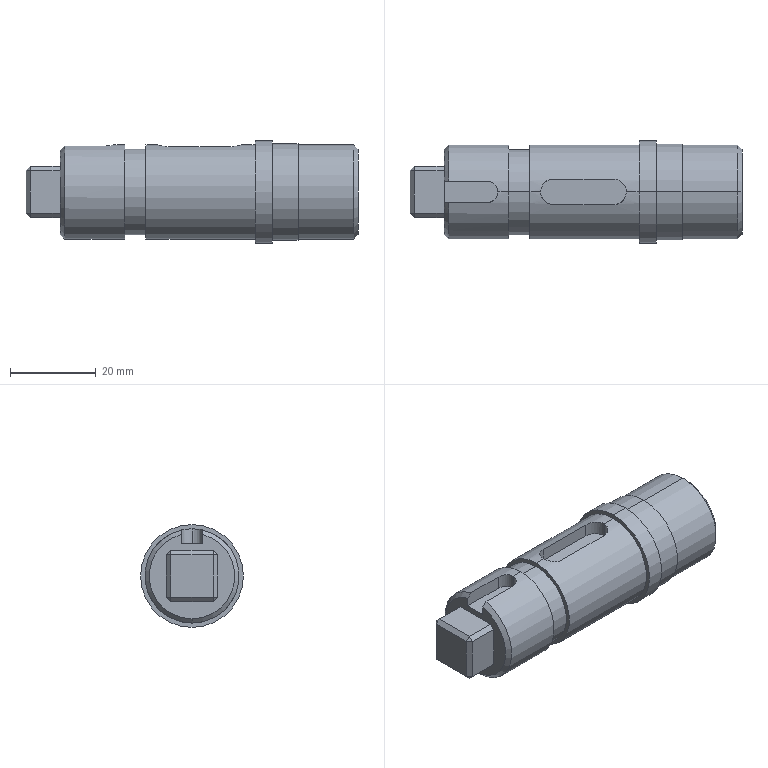Part | SolidWorks | features ICE 3, Chamfer 1, Revolution 1 | 1 solid | 51 faces | box 77.5 x 24 x 24 mm | volume 26951 mm3 | plane 30 | cylinder 17 | cone 4 | commonest cylinder face diameters 22 x6 6 x3 5 x2 20 x2 22.5 x2 24 x2
STEP:
#1=CARTESIAN_POINT('',(-28.866,0.,7.5));
#2=VERTEX_POINT('',#1);
#3=CARTESIAN_POINT('',(-31.366,2.5,7.5));
#4=VERTEX_POINT('',#3);
#5=CARTESIAN_POINT('',(-31.366,0.,7.5));
#6=DIRECTION('',(0.,0.,1.));
#7=DIRECTION('',(1.,0.,0.));
#8=AXIS2_PLACEMENT_3D('',#5,#6,#7);
#9=CIRCLE('',#8,2.5);
#10=EDGE_CURVE('',#2,#4,#9,.T.);
#11=ORIENTED_EDGE('',*,*,#10,.F.);
#12=CARTESIAN_POINT('',(-28.866,0.,11.));
#13=VERTEX_POINT('',#12);
#14=CARTESIAN_POINT('',(-28.866,0.,7.5));
#15=DIRECTION('',(0.,0.,1.));
#16=VECTOR('',#15,1000.);
#17=LINE('',#14,#16);
#18=EDGE_CURVE('',#2,#13,#17,.T.);
#19=ORIENTED_EDGE('',*,*,#18,.T.);
#20=CARTESIAN_POINT('',(-31.366,2.5,10.712));
#21=VERTEX_POINT('',#20);
#22=CARTESIAN_POINT('',(-31.366,2.5,10.712));
#23=CARTESIAN_POINT('',(-31.2,2.5,10.712));
#24=CARTESIAN_POINT('',(-31.037,2.484,10.716));
#25=CARTESIAN_POINT('',(-30.717,2.42,10.731));
#26=CARTESIAN_POINT('',(-30.558,2.371,10.742));
#27=CARTESIAN_POINT('',(-30.255,2.246,10.769));
#28=CARTESIAN_POINT('',(-30.112,2.169,10.784));
#29=CARTESIAN_POINT('',(-29.84,1.987,10.819));
#30=CARTESIAN_POINT('',(-29.712,1.882,10.838));
#31=CARTESIAN_POINT('',(-29.367,1.537,10.895));
#32=CARTESIAN_POINT('',(-29.181,1.259,10.932));
#33=CARTESIAN_POINT('',(-28.994,0.8077,10.971));
#34=CARTESIAN_POINT('',(-28.946,0.6494,10.982));
#35=CARTESIAN_POINT('',(-28.882,0.3264,10.996));
#36=CARTESIAN_POINT('',(-28.866,0.1637,11.));
#37=CARTESIAN_POINT('',(-28.866,0.,11.));
#38=B_SPLINE_CURVE_WITH_KNOTS('',3,(#22,#23,#24,#25,#26,#27,#28,#29,#30,#31,#32,#33,#34,#35,#36,#37),.UNSPECIFIED.,.F.,.F.,(4,2,2,2,2,2,2,4),(0.,0.0004902,0.0009805,0.001471,0.001961,0.002941,0.003432,0.003922),.UNSPECIFIED.);
#39=EDGE_CURVE('',#21,#13,#38,.T.);
#40=ORIENTED_EDGE('',*,*,#39,.F.);
#41=CARTESIAN_POINT('',(-31.366,2.5,7.5));
#42=DIRECTION('',(0.,0.,1.));
#43=VECTOR('',#42,1000.);
#44=LINE('',#41,#43);
#45=EDGE_CURVE('',#4,#21,#44,.T.);
#46=ORIENTED_EDGE('',*,*,#45,.F.);
#47=EDGE_LOOP('',(#11,#19,#40,#46));
#48=FACE_OUTER_BOUND('',#47,.T.);
#49=CARTESIAN_POINT('',(-31.366,0.,7.5));
#50=DIRECTION('',(0.,0.,1.));
#51=DIRECTION('',(1.,0.,0.));
#52=AXIS2_PLACEMENT_3D('',#49,#50,#51);
#53=CYLINDRICAL_SURFACE('',#52,2.5);
#54=ADVANCED_FACE('',(#48),#53,.F.);
#55=CARTESIAN_POINT('',(1.134,0.,7.5));
#56=VERTEX_POINT('',#55);
#57=CARTESIAN_POINT('',(-1.866,3.,7.5));
#58=VERTEX_POINT('',#57);
#59=CARTESIAN_POINT('',(-1.866,0.,7.5));
#60=DIRECTION('',(0.,0.,1.));
#61=DIRECTION('',(1.,0.,0.));
#62=AXIS2_PLACEMENT_3D('',#59,#60,#61);
#63=CIRCLE('',#62,3.);
#64=EDGE_CURVE('',#56,#58,#63,.T.);
#65=ORIENTED_EDGE('',*,*,#64,.F.);
#66=CARTESIAN_POINT('',(1.134,0.,11.));
#67=VERTEX_POINT('',#66);
#68=CARTESIAN_POINT('',(1.134,0.,7.5));
#69=DIRECTION('',(0.,0.,1.));
#70=VECTOR('',#69,1000.);
#71=LINE('',#68,#70);
#72=EDGE_CURVE('',#56,#67,#71,.T.);
#73=ORIENTED_EDGE('',*,*,#72,.T.);
#74=CARTESIAN_POINT('',(-1.866,3.,10.583));
#75=VERTEX_POINT('',#74);
#76=CARTESIAN_POINT('',(-1.866,3.,10.583));
#77=CARTESIAN_POINT('',(-1.666,3.,10.583));
#78=CARTESIAN_POINT('',(-1.471,2.98,10.589));
#79=CARTESIAN_POINT('',(-1.086,2.903,10.61));
#80=CARTESIAN_POINT('',(-0.8948,2.845,10.626));
#81=CARTESIAN_POINT('',(-0.5318,2.694,10.665));
#82=CARTESIAN_POINT('',(-0.3599,2.602,10.688));
#83=CARTESIAN_POINT('',(-0.03443,2.384,10.739));
#84=CARTESIAN_POINT('',(0.1189,2.258,10.767));
#85=CARTESIAN_POINT('',(0.3941,1.983,10.821));
#86=CARTESIAN_POINT('',(0.518,1.832,10.848));
#87=CARTESIAN_POINT('',(0.7374,1.504,10.898));
#88=CARTESIAN_POINT('',(0.8299,1.331,10.921));
#89=CARTESIAN_POINT('',(0.9797,0.9703,10.959));
#90=CARTESIAN_POINT('',(1.038,0.78,10.974));
#91=CARTESIAN_POINT('',(1.115,0.3922,10.995));
#92=CARTESIAN_POINT('',(1.134,0.1968,11.));
#93=CARTESIAN_POINT('',(1.134,0.,11.));
#94=B_SPLINE_CURVE_WITH_KNOTS('',3,(#76,#77,#78,#79,#80,#81,#82,#83,#84,#85,#86,#87,#88,#89,#90,#91,#92,#93),.UNSPECIFIED.,.F.,.F.,(4,2,2,2,2,2,2,2,4),(0.,0.0005892,0.001178,0.001767,0.002357,0.002946,0.003535,0.004124,0.004713),.UNSPECIFIED.);
#95=EDGE_CURVE('',#75,#67,#94,.T.);
#96=ORIENTED_EDGE('',*,*,#95,.F.);
#97=CARTESIAN_POINT('',(-1.866,3.,7.5));
#98=DIRECTION('',(0.,0.,1.));
#99=VECTOR('',#98,1000.);
#100=LINE('',#97,#99);
#101=EDGE_CURVE('',#58,#75,#100,.T.);
#102=ORIENTED_EDGE('',*,*,#101,.F.);
#103=EDGE_LOOP('',(#65,#73,#96,#102));
#104=FACE_OUTER_BOUND('',#103,.T.);
#105=CARTESIAN_POINT('',(-1.866,0.,7.5));
#106=DIRECTION('',(0.,0.,1.));
#107=DIRECTION('',(1.,0.,0.));
#108=AXIS2_PLACEMENT_3D('',#105,#106,#107);
#109=CYLINDRICAL_SURFACE('',#108,3.);
#110=ADVANCED_FACE('',(#104),#109,.F.);
#111=CARTESIAN_POINT('',(-41.366,0.,-10.));
#112=VERTEX_POINT('',#111);
#113=CARTESIAN_POINT('',(-41.366,-2.5,9.682));
#114=VERTEX_POINT('',#113);
#115=CARTESIAN_POINT('',(-41.366,0.,0.));
#116=DIRECTION('',(-1.,0.,0.));
#117=DIRECTION('',(0.,0.,-1.));
#118=AXIS2_PLACEMENT_3D('',#115,#116,#117);
#119=CIRCLE('',#118,10.);
#120=EDGE_CURVE('',#112,#114,#119,.T.);
#121=ORIENTED_EDGE('',*,*,#120,.F.);
#122=CARTESIAN_POINT('',(-40.366,0.,-11.));
#123=VERTEX_POINT('',#122);
#124=CARTESIAN_POINT('',(-41.366,0.,-10.));
#125=DIRECTION('',(0.7071,0.,-0.7071));
#126=VECTOR('',#125,1000.);
#127=LINE('',#124,#126);
#128=EDGE_CURVE('',#112,#123,#127,.T.);
#129=ORIENTED_EDGE('',*,*,#128,.T.);
#130=CARTESIAN_POINT('',(-40.366,-2.5,10.712));
#131=VERTEX_POINT('',#130);
#132=CARTESIAN_POINT('',(-40.366,0.,0.));
#133=DIRECTION('',(1.,0.,0.));
#134=DIRECTION('',(0.,0.,-1.));
#135=AXIS2_PLACEMENT_3D('',#132,#133,#134);
#136=CIRCLE('',#135,11.);
#137=EDGE_CURVE('',#131,#123,#136,.T.);
#138=ORIENTED_EDGE('',*,*,#137,.F.);
#139=CARTESIAN_POINT('',(-41.366,-2.5,9.682));
#140=CARTESIAN_POINT('',(-41.033,-2.5,10.026));
#141=CARTESIAN_POINT('',(-40.7,-2.5,10.369));
#142=CARTESIAN_POINT('',(-40.366,-2.5,10.712));
#143=B_SPLINE_CURVE_WITH_KNOTS('',3,(#139,#140,#141,#142),.UNSPECIFIED.,.F.,.F.,(4,4),(0.005287,0.006723),.UNSPECIFIED.);
#144=EDGE_CURVE('',#114,#131,#143,.T.);
#145=ORIENTED_EDGE('',*,*,#144,.F.);
#146=EDGE_LOOP('',(#121,#129,#138,#145));
#147=FACE_OUTER_BOUND('',#146,.T.);
#148=CARTESIAN_POINT('',(-41.366,0.,0.));
#149=DIRECTION('',(1.,0.,0.));
#150=DIRECTION('',(0.,0.,-1.));
#151=AXIS2_PLACEMENT_3D('',#148,#149,#150);
#152=CONICAL_SURFACE('',#151,10.,0.7854);
#153=ADVANCED_FACE('',(#147),#152,.T.);
#154=CARTESIAN_POINT('',(28.134,0.,-10.));
#155=VERTEX_POINT('',#154);
#156=CARTESIAN_POINT('',(28.134,0.,10.));
#157=VERTEX_POINT('',#156);
#158=CARTESIAN_POINT('',(28.134,0.,0.));
#159=DIRECTION('',(1.,0.,0.));
#160=DIRECTION('',(0.,0.,1.));
#161=AXIS2_PLACEMENT_3D('',#158,#159,#160);
#162=CIRCLE('',#161,10.);
#163=EDGE_CURVE('',#155,#157,#162,.T.);
#164=ORIENTED_EDGE('',*,*,#163,.F.);
#165=CARTESIAN_POINT('',(27.134,0.,-11.));
#166=VERTEX_POINT('',#165);
#167=CARTESIAN_POINT('',(27.134,0.,-11.));
#168=DIRECTION('',(-0.7071,0.,-0.7071));
#169=VECTOR('',#168,1000.);
#170=LINE('',#167,#169);
#171=EDGE_CURVE('',#155,#166,#170,.T.);
#172=ORIENTED_EDGE('',*,*,#171,.T.);
#173=CARTESIAN_POINT('',(27.134,0.,11.));
#174=VERTEX_POINT('',#173);
#175=CARTESIAN_POINT('',(27.134,0.,0.));
#176=DIRECTION('',(-1.,0.,0.));
#177=DIRECTION('',(0.,0.,1.));
#178=AXIS2_PLACEMENT_3D('',#175,#176,#177);
#179=CIRCLE('',#178,11.);
#180=EDGE_CURVE('',#174,#166,#179,.T.);
#181=ORIENTED_EDGE('',*,*,#180,.F.);
#182=CARTESIAN_POINT('',(27.134,0.,11.));
#183=DIRECTION('',(-0.7071,0.,0.7071));
#184=VECTOR('',#183,1000.);
#185=LINE('',#182,#184);
#186=EDGE_CURVE('',#157,#174,#185,.T.);
#187=ORIENTED_EDGE('',*,*,#186,.F.);
#188=EDGE_LOOP('',(#164,#172,#181,#187));
#189=FACE_OUTER_BOUND('',#188,.T.);
#190=CARTESIAN_POINT('',(27.134,0.,0.));
#191=DIRECTION('',(-1.,0.,0.));
#192=DIRECTION('',(0.,0.,1.));
#193=AXIS2_PLACEMENT_3D('',#190,#191,#192);
#194=CONICAL_SURFACE('',#193,11.,0.7854);
#195=ADVANCED_FACE('',(#189),#194,.T.);
#196=CARTESIAN_POINT('',(-26.366,0.,11.));
#197=VERTEX_POINT('',#196);
#198=CARTESIAN_POINT('',(-26.366,0.,-11.));
#199=VERTEX_POINT('',#198);
#200=CARTESIAN_POINT('',(-26.366,0.,0.));
#201=DIRECTION('',(-1.,0.,0.));
#202=DIRECTION('',(0.,0.,1.));
#203=AXIS2_PLACEMENT_3D('',#200,#201,#202);
#204=CIRCLE('',#203,11.);
#205=EDGE_CURVE('',#197,#199,#204,.T.);
#206=ORIENTED_EDGE('',*,*,#205,.T.);
#207=CARTESIAN_POINT('',(-41.366,0.,-11.));
#208=DIRECTION('',(-1.,0.,0.));
#209=VECTOR('',#208,1000.);
#210=LINE('',#207,#209);
#211=EDGE_CURVE('',#199,#123,#210,.T.);
#212=ORIENTED_EDGE('',*,*,#211,.T.);
#213=CARTESIAN_POINT('',(-40.366,2.5,10.712));
#214=VERTEX_POINT('',#213);
#215=CARTESIAN_POINT('',(-40.366,0.,0.));
#216=DIRECTION('',(1.,0.,0.));
#217=DIRECTION('',(0.,0.,-1.));
#218=AXIS2_PLACEMENT_3D('',#215,#216,#217);
#219=CIRCLE('',#218,11.);
#220=EDGE_CURVE('',#123,#214,#219,.T.);
#221=ORIENTED_EDGE('',*,*,#220,.T.);
#222=CARTESIAN_POINT('',(-41.366,2.5,10.712));
#223=DIRECTION('',(1.,0.,0.));
#224=VECTOR('',#223,1000.);
#225=LINE('',#222,#224);
#226=EDGE_CURVE('',#214,#21,#225,.T.);
#227=ORIENTED_EDGE('',*,*,#226,.T.);
#228=ORIENTED_EDGE('',*,*,#39,.T.);
#229=CARTESIAN_POINT('',(-41.366,0.,11.));
#230=DIRECTION('',(-1.,0.,0.));
#231=VECTOR('',#230,1000.);
#232=LINE('',#229,#231);
#233=EDGE_CURVE('',#197,#13,#232,.T.);
#234=ORIENTED_EDGE('',*,*,#233,.F.);
#235=EDGE_LOOP('',(#206,#212,#221,#227,#228,#234));
#236=FACE_OUTER_BOUND('',#235,.T.);
#237=CARTESIAN_POINT('',(-41.366,0.,0.));
#238=DIRECTION('',(-1.,0.,0.));
#239=DIRECTION('',(0.,0.,1.));
#240=AXIS2_PLACEMENT_3D('',#237,#238,#239);
#241=CYLINDRICAL_SURFACE('',#240,11.);
#242=ADVANCED_FACE('',(#236),#241,.T.);
#243=CARTESIAN_POINT('',(-21.366,0.,10.));
#244=VERTEX_POINT('',#243);
#245=CARTESIAN_POINT('',(-21.366,0.,-10.));
#246=VERTEX_POINT('',#245);
#247=CARTESIAN_POINT('',(-21.366,0.,0.));
#248=DIRECTION('',(-1.,0.,0.));
#249=DIRECTION('',(0.,0.,1.));
#250=AXIS2_PLACEMENT_3D('',#247,#248,#249);
#251=CIRCLE('',#250,10.);
#252=EDGE_CURVE('',#244,#246,#251,.T.);
#253=ORIENTED_EDGE('',*,*,#252,.T.);
#254=CARTESIAN_POINT('',(-26.366,0.,-10.));
#255=VERTEX_POINT('',#254);
#256=CARTESIAN_POINT('',(-41.366,0.,-10.));
#257=DIRECTION('',(-1.,0.,0.));
#258=VECTOR('',#257,1000.);
#259=LINE('',#256,#258);
#260=EDGE_CURVE('',#246,#255,#259,.T.);
#261=ORIENTED_EDGE('',*,*,#260,.T.);
#262=CARTESIAN_POINT('',(-26.366,0.,10.));
#263=VERTEX_POINT('',#262);
#264=CARTESIAN_POINT('',(-26.366,0.,0.));
#265=DIRECTION('',(-1.,0.,0.));
#266=DIRECTION('',(0.,0.,1.));
#267=AXIS2_PLACEMENT_3D('',#264,#265,#266);
#268=CIRCLE('',#267,10.);
#269=EDGE_CURVE('',#263,#255,#268,.T.);
#270=ORIENTED_EDGE('',*,*,#269,.F.);
#271=CARTESIAN_POINT('',(-41.366,0.,10.));
#272=DIRECTION('',(-1.,0.,0.));
#273=VECTOR('',#272,1000.);
#274=LINE('',#271,#273);
#275=EDGE_CURVE('',#244,#263,#274,.T.);
#276=ORIENTED_EDGE('',*,*,#275,.F.);
#277=EDGE_LOOP('',(#253,#261,#270,#276));
#278=FACE_OUTER_BOUND('',#277,.T.);
#279=CARTESIAN_POINT('',(-41.366,0.,0.));
#280=DIRECTION('',(-1.,0.,0.));
#281=DIRECTION('',(0.,0.,1.));
#282=AXIS2_PLACEMENT_3D('',#279,#280,#281);
#283=CYLINDRICAL_SURFACE('',#282,10.);
#284=ADVANCED_FACE('',(#278),#283,.T.);
#285=CARTESIAN_POINT('',(4.134,0.,11.));
#286=VERTEX_POINT('',#285);
#287=CARTESIAN_POINT('',(4.134,0.,-11.));
#288=VERTEX_POINT('',#287);
#289=CARTESIAN_POINT('',(4.134,0.,0.));
#290=DIRECTION('',(-1.,0.,0.));
#291=DIRECTION('',(0.,0.,1.));
#292=AXIS2_PLACEMENT_3D('',#289,#290,#291);
#293=CIRCLE('',#292,11.);
#294=EDGE_CURVE('',#286,#288,#293,.T.);
#295=ORIENTED_EDGE('',*,*,#294,.T.);
#296=CARTESIAN_POINT('',(-21.366,0.,-11.));
#297=VERTEX_POINT('',#296);
#298=CARTESIAN_POINT('',(-41.366,0.,-11.));
#299=DIRECTION('',(-1.,0.,0.));
#300=VECTOR('',#299,1000.);
#301=LINE('',#298,#300);
#302=EDGE_CURVE('',#288,#297,#301,.T.);
#303=ORIENTED_EDGE('',*,*,#302,.T.);
#304=CARTESIAN_POINT('',(-21.366,0.,11.));
#305=VERTEX_POINT('',#304);
#306=CARTESIAN_POINT('',(-21.366,0.,0.));
#307=DIRECTION('',(-1.,0.,0.));
#308=DIRECTION('',(0.,0.,1.));
#309=AXIS2_PLACEMENT_3D('',#306,#307,#308);
#310=CIRCLE('',#309,11.);
#311=EDGE_CURVE('',#305,#297,#310,.T.);
#312=ORIENTED_EDGE('',*,*,#311,.F.);
#313=CARTESIAN_POINT('',(-18.866,0.,11.));
#314=VERTEX_POINT('',#313);
#315=CARTESIAN_POINT('',(-41.366,0.,11.));
#316=DIRECTION('',(-1.,0.,0.));
#317=VECTOR('',#316,1000.);
#318=LINE('',#315,#317);
#319=EDGE_CURVE('',#314,#305,#318,.T.);
#320=ORIENTED_EDGE('',*,*,#319,.F.);
#321=CARTESIAN_POINT('',(-15.866,3.,10.583));
#322=VERTEX_POINT('',#321);
#323=CARTESIAN_POINT('',(-18.866,0.,11.));
#324=CARTESIAN_POINT('',(-18.866,0.1966,11.));
#325=CARTESIAN_POINT('',(-18.846,0.3963,10.995));
#326=CARTESIAN_POINT('',(-18.769,0.7814,10.974));
#327=CARTESIAN_POINT('',(-18.712,0.9688,10.959));
#328=CARTESIAN_POINT('',(-18.485,1.515,10.901));
#329=CARTESIAN_POINT('',(-18.264,1.844,10.848));
#330=CARTESIAN_POINT('',(-17.848,2.26,10.766));
#331=CARTESIAN_POINT('',(-17.698,2.383,10.739));
#332=CARTESIAN_POINT('',(-17.374,2.601,10.689));
#333=CARTESIAN_POINT('',(-17.199,2.695,10.665));
#334=CARTESIAN_POINT('',(-16.837,2.845,10.626));
#335=CARTESIAN_POINT('',(-16.65,2.902,10.61));
#336=CARTESIAN_POINT('',(-16.264,2.98,10.589));
#337=CARTESIAN_POINT('',(-16.065,3.,10.583));
#338=CARTESIAN_POINT('',(-15.866,3.,10.583));
#339=B_SPLINE_CURVE_WITH_KNOTS('',3,(#323,#324,#325,#326,#327,#328,#329,#330,#331,#332,#333,#334,#335,#336,#337,#338),.UNSPECIFIED.,.F.,.F.,(4,2,2,2,2,2,2,4),(0.004713,0.005302,0.00589,0.007067,0.007656,0.008244,0.008833,0.009421),.UNSPECIFIED.);
#340=EDGE_CURVE('',#314,#322,#339,.T.);
#341=ORIENTED_EDGE('',*,*,#340,.T.);
#342=CARTESIAN_POINT('',(-41.366,3.,10.583));
#343=DIRECTION('',(1.,0.,0.));
#344=VECTOR('',#343,1000.);
#345=LINE('',#342,#344);
#346=EDGE_CURVE('',#322,#75,#345,.T.);
#347=ORIENTED_EDGE('',*,*,#346,.T.);
#348=ORIENTED_EDGE('',*,*,#95,.T.);
#349=CARTESIAN_POINT('',(-41.366,0.,11.));
#350=DIRECTION('',(-1.,0.,0.));
#351=VECTOR('',#350,1000.);
#352=LINE('',#349,#351);
#353=EDGE_CURVE('',#286,#67,#352,.T.);
#354=ORIENTED_EDGE('',*,*,#353,.F.);
#355=EDGE_LOOP('',(#295,#303,#312,#320,#341,#347,#348,#354));
#356=FACE_OUTER_BOUND('',#355,.T.);
#357=CARTESIAN_POINT('',(-41.366,0.,0.));
#358=DIRECTION('',(-1.,0.,0.));
#359=DIRECTION('',(0.,0.,1.));
#360=AXIS2_PLACEMENT_3D('',#357,#358,#359);
#361=CYLINDRICAL_SURFACE('',#360,11.);
#362=ADVANCED_FACE('',(#356),#361,.T.);
#363=CARTESIAN_POINT('',(8.134,0.,12.));
#364=VERTEX_POINT('',#363);
#365=CARTESIAN_POINT('',(8.134,0.,-12.));
#366=VERTEX_POINT('',#365);
#367=CARTESIAN_POINT('',(8.134,0.,0.));
#368=DIRECTION('',(-1.,0.,0.));
#369=DIRECTION('',(0.,0.,1.));
#370=AXIS2_PLACEMENT_3D('',#367,#368,#369);
#371=CIRCLE('',#370,12.);
#372=EDGE_CURVE('',#364,#366,#371,.T.);
#373=ORIENTED_EDGE('',*,*,#372,.T.);
#374=CARTESIAN_POINT('',(4.134,0.,-12.));
#375=VERTEX_POINT('',#374);
#376=CARTESIAN_POINT('',(-41.366,0.,-12.));
#377=DIRECTION('',(-1.,0.,0.));
#378=VECTOR('',#377,1000.);
#379=LINE('',#376,#378);
#380=EDGE_CURVE('',#366,#375,#379,.T.);
#381=ORIENTED_EDGE('',*,*,#380,.T.);
#382=CARTESIAN_POINT('',(4.134,0.,12.));
#383=VERTEX_POINT('',#382);
#384=CARTESIAN_POINT('',(4.134,0.,0.));
#385=DIRECTION('',(-1.,0.,0.));
#386=DIRECTION('',(0.,0.,1.));
#387=AXIS2_PLACEMENT_3D('',#384,#385,#386);
#388=CIRCLE('',#387,12.);
#389=EDGE_CURVE('',#383,#375,#388,.T.);
#390=ORIENTED_EDGE('',*,*,#389,.F.);
#391=CARTESIAN_POINT('',(-41.366,0.,12.));
#392=DIRECTION('',(-1.,0.,0.));
#393=VECTOR('',#392,1000.);
#394=LINE('',#391,#393);
#395=EDGE_CURVE('',#364,#383,#394,.T.);
#396=ORIENTED_EDGE('',*,*,#395,.F.);
#397=EDGE_LOOP('',(#373,#381,#390,#396));
#398=FACE_OUTER_BOUND('',#397,.T.);
#399=CARTESIAN_POINT('',(-41.366,0.,0.));
#400=DIRECTION('',(-1.,0.,0.));
#401=DIRECTION('',(0.,0.,1.));
#402=AXIS2_PLACEMENT_3D('',#399,#400,#401);
#403=CYLINDRICAL_SURFACE('',#402,12.);
#404=ADVANCED_FACE('',(#398),#403,.T.);
#405=CARTESIAN_POINT('',(14.134,0.,11.25));
#406=VERTEX_POINT('',#405);
#407=CARTESIAN_POINT('',(14.134,0.,-11.25));
#408=VERTEX_POINT('',#407);
#409=CARTESIAN_POINT('',(14.134,0.,0.));
#410=DIRECTION('',(-1.,0.,0.));
#411=DIRECTION('',(0.,0.,1.));
#412=AXIS2_PLACEMENT_3D('',#409,#410,#411);
#413=CIRCLE('',#412,11.25);
#414=EDGE_CURVE('',#406,#408,#413,.T.);
#415=ORIENTED_EDGE('',*,*,#414,.T.);
#416=CARTESIAN_POINT('',(8.134,0.,-11.25));
#417=VERTEX_POINT('',#416);
#418=CARTESIAN_POINT('',(-41.366,0.,-11.25));
#419=DIRECTION('',(-1.,0.,0.));
#420=VECTOR('',#419,1000.);
#421=LINE('',#418,#420);
#422=EDGE_CURVE('',#408,#417,#421,.T.);
#423=ORIENTED_EDGE('',*,*,#422,.T.);
#424=CARTESIAN_POINT('',(8.134,0.,11.25));
#425=VERTEX_POINT('',#424);
#426=CARTESIAN_POINT('',(8.134,0.,0.));
#427=DIRECTION('',(-1.,0.,0.));
#428=DIRECTION('',(0.,0.,1.));
#429=AXIS2_PLACEMENT_3D('',#426,#427,#428);
#430=CIRCLE('',#429,11.25);
#431=EDGE_CURVE('',#425,#417,#430,.T.);
#432=ORIENTED_EDGE('',*,*,#431,.F.);
#433=CARTESIAN_POINT('',(-41.366,0.,11.25));
#434=DIRECTION('',(-1.,0.,0.));
#435=VECTOR('',#434,1000.);
#436=LINE('',#433,#435);
#437=EDGE_CURVE('',#406,#425,#436,.T.);
#438=ORIENTED_EDGE('',*,*,#437,.F.);
#439=EDGE_LOOP('',(#415,#423,#432,#438));
#440=FACE_OUTER_BOUND('',#439,.T.);
#441=CARTESIAN_POINT('',(-41.366,0.,0.));
#442=DIRECTION('',(-1.,0.,0.));
#443=DIRECTION('',(0.,0.,1.));
#444=AXIS2_PLACEMENT_3D('',#441,#442,#443);
#445=CYLINDRICAL_SURFACE('',#444,11.25);
#446=ADVANCED_FACE('',(#440),#445,.T.);
#447=ORIENTED_EDGE('',*,*,#180,.T.);
#448=CARTESIAN_POINT('',(14.134,0.,-11.));
#449=VERTEX_POINT('',#448);
#450=CARTESIAN_POINT('',(-41.366,0.,-11.));
#451=DIRECTION('',(-1.,0.,0.));
#452=VECTOR('',#451,1000.);
#453=LINE('',#450,#452);
#454=EDGE_CURVE('',#166,#449,#453,.T.);
#455=ORIENTED_EDGE('',*,*,#454,.T.);
#456=CARTESIAN_POINT('',(14.134,0.,11.));
#457=VERTEX_POINT('',#456);
#458=CARTESIAN_POINT('',(14.134,0.,0.));
#459=DIRECTION('',(-1.,0.,0.));
#460=DIRECTION('',(0.,0.,1.));
#461=AXIS2_PLACEMENT_3D('',#458,#459,#460);
#462=CIRCLE('',#461,11.);
#463=EDGE_CURVE('',#457,#449,#462,.T.);
#464=ORIENTED_EDGE('',*,*,#463,.F.);
#465=CARTESIAN_POINT('',(-41.366,0.,11.));
#466=DIRECTION('',(-1.,0.,0.));
#467=VECTOR('',#466,1000.);
#468=LINE('',#465,#467);
#469=EDGE_CURVE('',#174,#457,#468,.T.);
#470=ORIENTED_EDGE('',*,*,#469,.F.);
#471=EDGE_LOOP('',(#447,#455,#464,#470));
#472=FACE_OUTER_BOUND('',#471,.T.);
#473=CARTESIAN_POINT('',(-41.366,0.,0.));
#474=DIRECTION('',(-1.,0.,0.));
#475=DIRECTION('',(0.,0.,1.));
#476=AXIS2_PLACEMENT_3D('',#473,#474,#475);
#477=CYLINDRICAL_SURFACE('',#476,11.);
#478=ADVANCED_FACE('',(#472),#477,.T.);
#479=CARTESIAN_POINT('',(-41.366,2.5,9.682));
#480=VERTEX_POINT('',#479);
#481=CARTESIAN_POINT('',(-41.366,0.,0.));
#482=DIRECTION('',(-1.,0.,0.));
#483=DIRECTION('',(0.,0.,-1.));
#484=AXIS2_PLACEMENT_3D('',#481,#482,#483);
#485=CIRCLE('',#484,10.);
#486=EDGE_CURVE('',#480,#112,#485,.T.);
#487=ORIENTED_EDGE('',*,*,#486,.T.);
#488=ORIENTED_EDGE('',*,*,#120,.T.);
#489=CARTESIAN_POINT('',(-41.366,-2.5,7.5));
#490=VERTEX_POINT('',#489);
#491=CARTESIAN_POINT('',(-41.366,-2.5,7.5));
#492=DIRECTION('',(0.,0.,1.));
#493=VECTOR('',#492,1000.);
#494=LINE('',#491,#493);
#495=EDGE_CURVE('',#490,#114,#494,.T.);
#496=ORIENTED_EDGE('',*,*,#495,.F.);
#497=CARTESIAN_POINT('',(-41.366,2.5,7.5));
#498=VERTEX_POINT('',#497);
#499=CARTESIAN_POINT('',(-41.366,2.5,7.5));
#500=DIRECTION('',(0.,-1.,0.));
#501=VECTOR('',#500,1000.);
#502=LINE('',#499,#501);
#503=EDGE_CURVE('',#498,#490,#502,.T.);
#504=ORIENTED_EDGE('',*,*,#503,.F.);
#505=CARTESIAN_POINT('',(-41.366,2.5,7.5));
#506=DIRECTION('',(0.,0.,1.));
#507=VECTOR('',#506,1000.);
#508=LINE('',#505,#507);
#509=EDGE_CURVE('',#498,#480,#508,.T.);
#510=ORIENTED_EDGE('',*,*,#509,.T.);
#511=EDGE_LOOP('',(#487,#488,#496,#504,#510));
#512=FACE_OUTER_BOUND('',#511,.T.);
#513=CARTESIAN_POINT('',(-41.366,-5.,6.));
#514=VERTEX_POINT('',#513);
#515=CARTESIAN_POINT('',(-41.366,5.,6.));
#516=VERTEX_POINT('',#515);
#517=CARTESIAN_POINT('',(-41.366,-6.,6.));
#518=DIRECTION('',(0.,1.,0.));
#519=VECTOR('',#518,1000.);
#520=LINE('',#517,#519);
#521=EDGE_CURVE('',#514,#516,#520,.T.);
#522=ORIENTED_EDGE('',*,*,#521,.F.);
#523=CARTESIAN_POINT('',(-41.366,-6.,5.));
#524=VERTEX_POINT('',#523);
#525=CARTESIAN_POINT('',(-41.366,0.,11.));
#526=DIRECTION('',(0.,-0.7071,-0.7071));
#527=VECTOR('',#526,1000.);
#528=LINE('',#525,#527);
#529=EDGE_CURVE('',#514,#524,#528,.T.);
#530=ORIENTED_EDGE('',*,*,#529,.T.);
#531=CARTESIAN_POINT('',(-41.366,-6.,-5.));
#532=VERTEX_POINT('',#531);
#533=CARTESIAN_POINT('',(-41.366,-6.,-6.));
#534=DIRECTION('',(0.,0.,1.));
#535=VECTOR('',#534,1000.);
#536=LINE('',#533,#535);
#537=EDGE_CURVE('',#532,#524,#536,.T.);
#538=ORIENTED_EDGE('',*,*,#537,.F.);
#539=CARTESIAN_POINT('',(-41.366,-5.,-6.));
#540=VERTEX_POINT('',#539);
#541=CARTESIAN_POINT('',(-41.366,0.,-11.));
#542=DIRECTION('',(0.,0.7071,-0.7071));
#543=VECTOR('',#542,1000.);
#544=LINE('',#541,#543);
#545=EDGE_CURVE('',#532,#540,#544,.T.);
#546=ORIENTED_EDGE('',*,*,#545,.T.);
#547=CARTESIAN_POINT('',(-41.366,5.,-6.));
#548=VERTEX_POINT('',#547);
#549=CARTESIAN_POINT('',(-41.366,-6.,-6.));
#550=DIRECTION('',(0.,-1.,0.));
#551=VECTOR('',#550,1000.);
#552=LINE('',#549,#551);
#553=EDGE_CURVE('',#548,#540,#552,.T.);
#554=ORIENTED_EDGE('',*,*,#553,.F.);
#555=CARTESIAN_POINT('',(-41.366,6.,-5.));
#556=VERTEX_POINT('',#555);
#557=CARTESIAN_POINT('',(-41.366,11.,0.));
#558=DIRECTION('',(0.,0.7071,0.7071));
#559=VECTOR('',#558,1000.);
#560=LINE('',#557,#559);
#561=EDGE_CURVE('',#548,#556,#560,.T.);
#562=ORIENTED_EDGE('',*,*,#561,.T.);
#563=CARTESIAN_POINT('',(-41.366,6.,5.));
#564=VERTEX_POINT('',#563);
#565=CARTESIAN_POINT('',(-41.366,6.,-6.));
#566=DIRECTION('',(0.,0.,-1.));
#567=VECTOR('',#566,1000.);
#568=LINE('',#565,#567);
#569=EDGE_CURVE('',#564,#556,#568,.T.);
#570=ORIENTED_EDGE('',*,*,#569,.F.);
#571=CARTESIAN_POINT('',(-41.366,11.,0.));
#572=DIRECTION('',(0.,-0.7071,0.7071));
#573=VECTOR('',#572,1000.);
#574=LINE('',#571,#573);
#575=EDGE_CURVE('',#564,#516,#574,.T.);
#576=ORIENTED_EDGE('',*,*,#575,.T.);
#577=EDGE_LOOP('',(#522,#530,#538,#546,#554,#562,#570,#576));
#578=FACE_BOUND('',#577,.T.);
#579=CARTESIAN_POINT('',(-41.366,11.,0.));
#580=DIRECTION('',(1.,0.,0.));
#581=DIRECTION('',(0.,0.,-1.));
#582=AXIS2_PLACEMENT_3D('',#579,#580,#581);
#583=PLANE('',#582);
#584=ADVANCED_FACE('',(#512,#578),#583,.F.);
#585=CARTESIAN_POINT('',(28.134,0.,0.));
#586=DIRECTION('',(1.,0.,0.));
#587=DIRECTION('',(0.,0.,1.));
#588=AXIS2_PLACEMENT_3D('',#585,#586,#587);
#589=CIRCLE('',#588,10.);
#590=EDGE_CURVE('',#157,#155,#589,.T.);
#591=ORIENTED_EDGE('',*,*,#590,.T.);
#592=ORIENTED_EDGE('',*,*,#163,.T.);
#593=EDGE_LOOP('',(#591,#592));
#594=FACE_OUTER_BOUND('',#593,.T.);
#595=CARTESIAN_POINT('',(28.134,0.,0.));
#596=DIRECTION('',(-1.,0.,0.));
#597=DIRECTION('',(0.,0.,1.));
#598=AXIS2_PLACEMENT_3D('',#595,#596,#597);
#599=PLANE('',#598);
#600=ADVANCED_FACE('',(#594),#599,.F.);
#601=ORIENTED_EDGE('',*,*,#454,.F.);
#602=CARTESIAN_POINT('',(27.134,0.,0.));
#603=DIRECTION('',(-1.,0.,0.));
#604=DIRECTION('',(0.,0.,1.));
#605=AXIS2_PLACEMENT_3D('',#602,#603,#604);
#606=CIRCLE('',#605,11.);
#607=EDGE_CURVE('',#166,#174,#606,.T.);
#608=ORIENTED_EDGE('',*,*,#607,.T.);
#609=ORIENTED_EDGE('',*,*,#469,.T.);
#610=CARTESIAN_POINT('',(14.134,0.,0.));
#611=DIRECTION('',(-1.,0.,0.));
#612=DIRECTION('',(0.,0.,1.));
#613=AXIS2_PLACEMENT_3D('',#610,#611,#612);
#614=CIRCLE('',#613,11.);
#615=EDGE_CURVE('',#449,#457,#614,.T.);
#616=ORIENTED_EDGE('',*,*,#615,.F.);
#617=EDGE_LOOP('',(#601,#608,#609,#616));
#618=FACE_OUTER_BOUND('',#617,.T.);
#619=CARTESIAN_POINT('',(-41.366,0.,0.));
#620=DIRECTION('',(-1.,0.,0.));
#621=DIRECTION('',(0.,0.,1.));
#622=AXIS2_PLACEMENT_3D('',#619,#620,#621);
#623=CYLINDRICAL_SURFACE('',#622,11.);
#624=ADVANCED_FACE('',(#618),#623,.T.);
#625=ORIENTED_EDGE('',*,*,#414,.F.);
#626=CARTESIAN_POINT('',(14.134,0.,0.));
#627=DIRECTION('',(-1.,0.,0.));
#628=DIRECTION('',(0.,0.,1.));
#629=AXIS2_PLACEMENT_3D('',#626,#627,#628);
#630=CIRCLE('',#629,11.25);
#631=EDGE_CURVE('',#408,#406,#630,.T.);
#632=ORIENTED_EDGE('',*,*,#631,.F.);
#633=EDGE_LOOP('',(#625,#632));
#634=FACE_OUTER_BOUND('',#633,.T.);
#635=ORIENTED_EDGE('',*,*,#463,.T.);
#636=ORIENTED_EDGE('',*,*,#615,.T.);
#637=EDGE_LOOP('',(#635,#636));
#638=FACE_BOUND('',#637,.T.);
#639=CARTESIAN_POINT('',(14.134,11.,0.));
#640=DIRECTION('',(-1.,0.,0.));
#641=DIRECTION('',(0.,0.,1.));
#642=AXIS2_PLACEMENT_3D('',#639,#640,#641);
#643=PLANE('',#642);
#644=ADVANCED_FACE('',(#634,#638),#643,.F.);
#645=ORIENTED_EDGE('',*,*,#422,.F.);
#646=ORIENTED_EDGE('',*,*,#631,.T.);
#647=ORIENTED_EDGE('',*,*,#437,.T.);
#648=CARTESIAN_POINT('',(8.134,0.,0.));
#649=DIRECTION('',(-1.,0.,0.));
#650=DIRECTION('',(0.,0.,1.));
#651=AXIS2_PLACEMENT_3D('',#648,#649,#650);
#652=CIRCLE('',#651,11.25);
#653=EDGE_CURVE('',#417,#425,#652,.T.);
#654=ORIENTED_EDGE('',*,*,#653,.F.);
#655=EDGE_LOOP('',(#645,#646,#647,#654));
#656=FACE_OUTER_BOUND('',#655,.T.);
#657=CARTESIAN_POINT('',(-41.366,0.,0.));
#658=DIRECTION('',(-1.,0.,0.));
#659=DIRECTION('',(0.,0.,1.));
#660=AXIS2_PLACEMENT_3D('',#657,#658,#659);
#661=CYLINDRICAL_SURFACE('',#660,11.25);
#662=ADVANCED_FACE('',(#656),#661,.T.);
#663=ORIENTED_EDGE('',*,*,#372,.F.);
#664=CARTESIAN_POINT('',(8.134,0.,0.));
#665=DIRECTION('',(-1.,0.,0.));
#666=DIRECTION('',(0.,0.,1.));
#667=AXIS2_PLACEMENT_3D('',#664,#665,#666);
#668=CIRCLE('',#667,12.);
#669=EDGE_CURVE('',#366,#364,#668,.T.);
#670=ORIENTED_EDGE('',*,*,#669,.F.);
#671=EDGE_LOOP('',(#663,#670));
#672=FACE_OUTER_BOUND('',#671,.T.);
#673=ORIENTED_EDGE('',*,*,#431,.T.);
#674=ORIENTED_EDGE('',*,*,#653,.T.);
#675=EDGE_LOOP('',(#673,#674));
#676=FACE_BOUND('',#675,.T.);
#677=CARTESIAN_POINT('',(8.134,11.25,0.));
#678=DIRECTION('',(-1.,0.,0.));
#679=DIRECTION('',(0.,0.,1.));
#680=AXIS2_PLACEMENT_3D('',#677,#678,#679);
#681=PLANE('',#680);
#682=ADVANCED_FACE('',(#672,#676),#681,.F.);
#683=ORIENTED_EDGE('',*,*,#380,.F.);
#684=ORIENTED_EDGE('',*,*,#669,.T.);
#685=ORIENTED_EDGE('',*,*,#395,.T.);
#686=CARTESIAN_POINT('',(4.134,0.,0.));
#687=DIRECTION('',(-1.,0.,0.));
#688=DIRECTION('',(0.,0.,1.));
#689=AXIS2_PLACEMENT_3D('',#686,#687,#688);
#690=CIRCLE('',#689,12.);
#691=EDGE_CURVE('',#375,#383,#690,.T.);
#692=ORIENTED_EDGE('',*,*,#691,.F.);
#693=EDGE_LOOP('',(#683,#684,#685,#692));
#694=FACE_OUTER_BOUND('',#693,.T.);
#695=CARTESIAN_POINT('',(-41.366,0.,0.));
#696=DIRECTION('',(-1.,0.,0.));
#697=DIRECTION('',(0.,0.,1.));
#698=AXIS2_PLACEMENT_3D('',#695,#696,#697);
#699=CYLINDRICAL_SURFACE('',#698,12.);
#700=ADVANCED_FACE('',(#694),#699,.T.);
#701=ORIENTED_EDGE('',*,*,#294,.F.);
#702=CARTESIAN_POINT('',(4.134,0.,0.));
#703=DIRECTION('',(-1.,0.,0.));
#704=DIRECTION('',(0.,0.,1.));
#705=AXIS2_PLACEMENT_3D('',#702,#703,#704);
#706=CIRCLE('',#705,11.);
#707=EDGE_CURVE('',#288,#286,#706,.T.);
#708=ORIENTED_EDGE('',*,*,#707,.F.);
#709=EDGE_LOOP('',(#701,#708));
#710=FACE_BOUND('',#709,.T.);
#711=ORIENTED_EDGE('',*,*,#389,.T.);
#712=ORIENTED_EDGE('',*,*,#691,.T.);
#713=EDGE_LOOP('',(#711,#712));
#714=FACE_OUTER_BOUND('',#713,.T.);
#715=CARTESIAN_POINT('',(4.134,12.,0.));
#716=DIRECTION('',(1.,0.,0.));
#717=DIRECTION('',(0.,0.,-1.));
#718=AXIS2_PLACEMENT_3D('',#715,#716,#717);
#719=PLANE('',#718);
#720=ADVANCED_FACE('',(#710,#714),#719,.F.);
#721=ORIENTED_EDGE('',*,*,#302,.F.);
#722=ORIENTED_EDGE('',*,*,#707,.T.);
#723=ORIENTED_EDGE('',*,*,#353,.T.);
#724=CARTESIAN_POINT('',(-1.866,-3.,10.583));
#725=VERTEX_POINT('',#724);
#726=CARTESIAN_POINT('',(1.134,0.,11.));
#727=CARTESIAN_POINT('',(1.134,-0.1966,11.));
#728=CARTESIAN_POINT('',(1.114,-0.3963,10.995));
#729=CARTESIAN_POINT('',(1.037,-0.7814,10.974));
#730=CARTESIAN_POINT('',(0.9804,-0.9688,10.959));
#731=CARTESIAN_POINT('',(0.7535,-1.515,10.901));
#732=CARTESIAN_POINT('',(0.5327,-1.844,10.848));
#733=CARTESIAN_POINT('',(0.1168,-2.26,10.766));
#734=CARTESIAN_POINT('',(-0.03353,-2.383,10.739));
#735=CARTESIAN_POINT('',(-0.3573,-2.601,10.689));
#736=CARTESIAN_POINT('',(-0.5328,-2.695,10.665));
#737=CARTESIAN_POINT('',(-0.8943,-2.845,10.626));
#738=CARTESIAN_POINT('',(-1.081,-2.902,10.61));
#739=CARTESIAN_POINT('',(-1.467,-2.98,10.589));
#740=CARTESIAN_POINT('',(-1.667,-3.,10.583));
#741=CARTESIAN_POINT('',(-1.866,-3.,10.583));
#742=B_SPLINE_CURVE_WITH_KNOTS('',3,(#726,#727,#728,#729,#730,#731,#732,#733,#734,#735,#736,#737,#738,#739,#740,#741),.UNSPECIFIED.,.F.,.F.,(4,2,2,2,2,2,2,4),(0.004713,0.005302,0.00589,0.007067,0.007656,0.008244,0.008833,0.009421),.UNSPECIFIED.);
#743=EDGE_CURVE('',#67,#725,#742,.T.);
#744=ORIENTED_EDGE('',*,*,#743,.T.);
#745=CARTESIAN_POINT('',(-15.866,-3.,10.583));
#746=VERTEX_POINT('',#745);
#747=CARTESIAN_POINT('',(-41.366,-3.,10.583));
#748=DIRECTION('',(-1.,0.,0.));
#749=VECTOR('',#748,1000.);
#750=LINE('',#747,#749);
#751=EDGE_CURVE('',#725,#746,#750,.T.);
#752=ORIENTED_EDGE('',*,*,#751,.T.);
#753=CARTESIAN_POINT('',(-15.866,-3.,10.583));
#754=CARTESIAN_POINT('',(-16.065,-3.,10.583));
#755=CARTESIAN_POINT('',(-16.261,-2.98,10.589));
#756=CARTESIAN_POINT('',(-16.646,-2.903,10.61));
#757=CARTESIAN_POINT('',(-16.837,-2.845,10.626));
#758=CARTESIAN_POINT('',(-17.2,-2.694,10.665));
#759=CARTESIAN_POINT('',(-17.372,-2.602,10.688));
#760=CARTESIAN_POINT('',(-17.697,-2.384,10.739));
#761=CARTESIAN_POINT('',(-17.85,-2.258,10.767));
#762=CARTESIAN_POINT('',(-18.126,-1.983,10.821));
#763=CARTESIAN_POINT('',(-18.249,-1.832,10.848));
#764=CARTESIAN_POINT('',(-18.469,-1.504,10.898));
#765=CARTESIAN_POINT('',(-18.561,-1.331,10.921));
#766=CARTESIAN_POINT('',(-18.711,-0.9703,10.959));
#767=CARTESIAN_POINT('',(-18.769,-0.78,10.974));
#768=CARTESIAN_POINT('',(-18.847,-0.3922,10.995));
#769=CARTESIAN_POINT('',(-18.866,-0.1968,11.));
#770=CARTESIAN_POINT('',(-18.866,0.,11.));
#771=B_SPLINE_CURVE_WITH_KNOTS('',3,(#753,#754,#755,#756,#757,#758,#759,#760,#761,#762,#763,#764,#765,#766,#767,#768,#769,#770),.UNSPECIFIED.,.F.,.F.,(4,2,2,2,2,2,2,2,4),(0.,0.0005892,0.001178,0.001767,0.002357,0.002946,0.003535,0.004124,0.004713),.UNSPECIFIED.);
#772=EDGE_CURVE('',#746,#314,#771,.T.);
#773=ORIENTED_EDGE('',*,*,#772,.T.);
#774=ORIENTED_EDGE('',*,*,#319,.T.);
#775=CARTESIAN_POINT('',(-21.366,0.,0.));
#776=DIRECTION('',(-1.,0.,0.));
#777=DIRECTION('',(0.,0.,1.));
#778=AXIS2_PLACEMENT_3D('',#775,#776,#777);
#779=CIRCLE('',#778,11.);
#780=EDGE_CURVE('',#297,#305,#779,.T.);
#781=ORIENTED_EDGE('',*,*,#780,.F.);
#782=EDGE_LOOP('',(#721,#722,#723,#744,#752,#773,#774,#781));
#783=FACE_OUTER_BOUND('',#782,.T.);
#784=CARTESIAN_POINT('',(-41.366,0.,0.));
#785=DIRECTION('',(-1.,0.,0.));
#786=DIRECTION('',(0.,0.,1.));
#787=AXIS2_PLACEMENT_3D('',#784,#785,#786);
#788=CYLINDRICAL_SURFACE('',#787,11.);
#789=ADVANCED_FACE('',(#783),#788,.T.);
#790=ORIENTED_EDGE('',*,*,#252,.F.);
#791=CARTESIAN_POINT('',(-21.366,0.,0.));
#792=DIRECTION('',(-1.,0.,0.));
#793=DIRECTION('',(0.,0.,1.));
#794=AXIS2_PLACEMENT_3D('',#791,#792,#793);
#795=CIRCLE('',#794,10.);
#796=EDGE_CURVE('',#246,#244,#795,.T.);
#797=ORIENTED_EDGE('',*,*,#796,.F.);
#798=EDGE_LOOP('',(#790,#797));
#799=FACE_BOUND('',#798,.T.);
#800=ORIENTED_EDGE('',*,*,#311,.T.);
#801=ORIENTED_EDGE('',*,*,#780,.T.);
#802=EDGE_LOOP('',(#800,#801));
#803=FACE_OUTER_BOUND('',#802,.T.);
#804=CARTESIAN_POINT('',(-21.366,11.,0.));
#805=DIRECTION('',(1.,0.,0.));
#806=DIRECTION('',(0.,0.,-1.));
#807=AXIS2_PLACEMENT_3D('',#804,#805,#806);
#808=PLANE('',#807);
#809=ADVANCED_FACE('',(#799,#803),#808,.F.);
#810=ORIENTED_EDGE('',*,*,#260,.F.);
#811=ORIENTED_EDGE('',*,*,#796,.T.);
#812=ORIENTED_EDGE('',*,*,#275,.T.);
#813=CARTESIAN_POINT('',(-26.366,0.,0.));
#814=DIRECTION('',(-1.,0.,0.));
#815=DIRECTION('',(0.,0.,1.));
#816=AXIS2_PLACEMENT_3D('',#813,#814,#815);
#817=CIRCLE('',#816,10.);
#818=EDGE_CURVE('',#255,#263,#817,.T.);
#819=ORIENTED_EDGE('',*,*,#818,.F.);
#820=EDGE_LOOP('',(#810,#811,#812,#819));
#821=FACE_OUTER_BOUND('',#820,.T.);
#822=CARTESIAN_POINT('',(-41.366,0.,0.));
#823=DIRECTION('',(-1.,0.,0.));
#824=DIRECTION('',(0.,0.,1.));
#825=AXIS2_PLACEMENT_3D('',#822,#823,#824);
#826=CYLINDRICAL_SURFACE('',#825,10.);
#827=ADVANCED_FACE('',(#821),#826,.T.);
#828=ORIENTED_EDGE('',*,*,#205,.F.);
#829=CARTESIAN_POINT('',(-26.366,0.,0.));
#830=DIRECTION('',(-1.,0.,0.));
#831=DIRECTION('',(0.,0.,1.));
#832=AXIS2_PLACEMENT_3D('',#829,#830,#831);
#833=CIRCLE('',#832,11.);
#834=EDGE_CURVE('',#199,#197,#833,.T.);
#835=ORIENTED_EDGE('',*,*,#834,.F.);
#836=EDGE_LOOP('',(#828,#835));
#837=FACE_OUTER_BOUND('',#836,.T.);
#838=ORIENTED_EDGE('',*,*,#269,.T.);
#839=ORIENTED_EDGE('',*,*,#818,.T.);
#840=EDGE_LOOP('',(#838,#839));
#841=FACE_BOUND('',#840,.T.);
#842=CARTESIAN_POINT('',(-26.366,10.,0.));
#843=DIRECTION('',(-1.,0.,0.));
#844=DIRECTION('',(0.,0.,1.));
#845=AXIS2_PLACEMENT_3D('',#842,#843,#844);
#846=PLANE('',#845);
#847=ADVANCED_FACE('',(#837,#841),#846,.F.);
#848=ORIENTED_EDGE('',*,*,#211,.F.);
#849=ORIENTED_EDGE('',*,*,#834,.T.);
#850=ORIENTED_EDGE('',*,*,#233,.T.);
#851=CARTESIAN_POINT('',(-31.366,-2.5,10.712));
#852=VERTEX_POINT('',#851);
#853=CARTESIAN_POINT('',(-28.866,0.,11.));
#854=CARTESIAN_POINT('',(-28.866,-0.1635,11.));
#855=CARTESIAN_POINT('',(-28.882,-0.3297,10.996));
#856=CARTESIAN_POINT('',(-28.946,-0.6505,10.982));
#857=CARTESIAN_POINT('',(-28.994,-0.8065,10.971));
#858=CARTESIAN_POINT('',(-29.182,-1.261,10.932));
#859=CARTESIAN_POINT('',(-29.366,-1.536,10.895));
#860=CARTESIAN_POINT('',(-29.714,-1.884,10.838));
#861=CARTESIAN_POINT('',(-29.839,-1.987,10.82));
#862=CARTESIAN_POINT('',(-30.109,-2.167,10.785));
#863=CARTESIAN_POINT('',(-30.256,-2.246,10.768));
#864=CARTESIAN_POINT('',(-30.557,-2.371,10.742));
#865=CARTESIAN_POINT('',(-30.713,-2.419,10.731));
#866=CARTESIAN_POINT('',(-31.034,-2.483,10.716));
#867=CARTESIAN_POINT('',(-31.2,-2.5,10.712));
#868=CARTESIAN_POINT('',(-31.366,-2.5,10.712));
#869=B_SPLINE_CURVE_WITH_KNOTS('',3,(#853,#854,#855,#856,#857,#858,#859,#860,#861,#862,#863,#864,#865,#866,#867,#868),.UNSPECIFIED.,.F.,.F.,(4,2,2,2,2,2,2,4),(0.003922,0.004412,0.004901,0.005881,0.00637,0.00686,0.00735,0.00784),.UNSPECIFIED.);
#870=EDGE_CURVE('',#13,#852,#869,.T.);
#871=ORIENTED_EDGE('',*,*,#870,.T.);
#872=CARTESIAN_POINT('',(-41.366,-2.5,10.712));
#873=DIRECTION('',(-1.,0.,0.));
#874=VECTOR('',#873,1000.);
#875=LINE('',#872,#874);
#876=EDGE_CURVE('',#852,#131,#875,.T.);
#877=ORIENTED_EDGE('',*,*,#876,.T.);
#878=ORIENTED_EDGE('',*,*,#137,.T.);
#879=EDGE_LOOP('',(#848,#849,#850,#871,#877,#878));
#880=FACE_OUTER_BOUND('',#879,.T.);
#881=CARTESIAN_POINT('',(-41.366,0.,0.));
#882=DIRECTION('',(-1.,0.,0.));
#883=DIRECTION('',(0.,0.,1.));
#884=AXIS2_PLACEMENT_3D('',#881,#882,#883);
#885=CYLINDRICAL_SURFACE('',#884,11.);
#886=ADVANCED_FACE('',(#880),#885,.T.);
#887=CARTESIAN_POINT('',(-48.366,5.,6.));
#888=VERTEX_POINT('',#887);
#889=CARTESIAN_POINT('',(-48.366,-5.,6.));
#890=VERTEX_POINT('',#889);
#891=CARTESIAN_POINT('',(-48.366,-6.,6.));
#892=DIRECTION('',(0.,-1.,0.));
#893=VECTOR('',#892,1000.);
#894=LINE('',#891,#893);
#895=EDGE_CURVE('',#888,#890,#894,.T.);
#896=ORIENTED_EDGE('',*,*,#895,.T.);
#897=CARTESIAN_POINT('',(-49.366,-5.,6.));
#898=DIRECTION('',(1.,0.,0.));
#899=VECTOR('',#898,1000.);
#900=LINE('',#897,#899);
#901=EDGE_CURVE('',#890,#514,#900,.T.);
#902=ORIENTED_EDGE('',*,*,#901,.T.);
#903=ORIENTED_EDGE('',*,*,#521,.T.);
#904=CARTESIAN_POINT('',(-49.366,5.,6.));
#905=DIRECTION('',(-1.,0.,0.));
#906=VECTOR('',#905,1000.);
#907=LINE('',#904,#906);
#908=EDGE_CURVE('',#516,#888,#907,.T.);
#909=ORIENTED_EDGE('',*,*,#908,.T.);
#910=EDGE_LOOP('',(#896,#902,#903,#909));
#911=FACE_OUTER_BOUND('',#910,.T.);
#912=CARTESIAN_POINT('',(-49.366,-6.,6.));
#913=DIRECTION('',(0.,0.,-1.));
#914=DIRECTION('',(-1.,0.,0.));
#915=AXIS2_PLACEMENT_3D('',#912,#913,#914);
#916=PLANE('',#915);
#917=ADVANCED_FACE('',(#911),#916,.F.);
#918=ORIENTED_EDGE('',*,*,#569,.T.);
#919=CARTESIAN_POINT('',(-48.366,6.,-5.));
#920=VERTEX_POINT('',#919);
#921=CARTESIAN_POINT('',(-49.366,6.,-5.));
#922=DIRECTION('',(-1.,0.,0.));
#923=VECTOR('',#922,1000.);
#924=LINE('',#921,#923);
#925=EDGE_CURVE('',#556,#920,#924,.T.);
#926=ORIENTED_EDGE('',*,*,#925,.T.);
#927=CARTESIAN_POINT('',(-48.366,6.,5.));
#928=VERTEX_POINT('',#927);
#929=CARTESIAN_POINT('',(-48.366,6.,-6.));
#930=DIRECTION('',(0.,0.,1.));
#931=VECTOR('',#930,1000.);
#932=LINE('',#929,#931);
#933=EDGE_CURVE('',#920,#928,#932,.T.);
#934=ORIENTED_EDGE('',*,*,#933,.T.);
#935=CARTESIAN_POINT('',(-49.366,6.,5.));
#936=DIRECTION('',(1.,0.,0.));
#937=VECTOR('',#936,1000.);
#938=LINE('',#935,#937);
#939=EDGE_CURVE('',#928,#564,#938,.T.);
#940=ORIENTED_EDGE('',*,*,#939,.T.);
#941=EDGE_LOOP('',(#918,#926,#934,#940));
#942=FACE_OUTER_BOUND('',#941,.T.);
#943=CARTESIAN_POINT('',(-49.366,6.,-6.));
#944=DIRECTION('',(0.,-1.,0.));
#945=DIRECTION('',(0.,0.,-1.));
#946=AXIS2_PLACEMENT_3D('',#943,#944,#945);
#947=PLANE('',#946);
#948=ADVANCED_FACE('',(#942),#947,.F.);
#949=ORIENTED_EDGE('',*,*,#553,.T.);
#950=CARTESIAN_POINT('',(-48.366,-5.,-6.));
#951=VERTEX_POINT('',#950);
#952=CARTESIAN_POINT('',(-49.366,-5.,-6.));
#953=DIRECTION('',(-1.,0.,0.));
#954=VECTOR('',#953,1000.);
#955=LINE('',#952,#954);
#956=EDGE_CURVE('',#540,#951,#955,.T.);
#957=ORIENTED_EDGE('',*,*,#956,.T.);
#958=CARTESIAN_POINT('',(-48.366,5.,-6.));
#959=VERTEX_POINT('',#958);
#960=CARTESIAN_POINT('',(-48.366,-6.,-6.));
#961=DIRECTION('',(0.,1.,0.));
#962=VECTOR('',#961,1000.);
#963=LINE('',#960,#962);
#964=EDGE_CURVE('',#951,#959,#963,.T.);
#965=ORIENTED_EDGE('',*,*,#964,.T.);
#966=CARTESIAN_POINT('',(-49.366,5.,-6.));
#967=DIRECTION('',(1.,0.,0.));
#968=VECTOR('',#967,1000.);
#969=LINE('',#966,#968);
#970=EDGE_CURVE('',#959,#548,#969,.T.);
#971=ORIENTED_EDGE('',*,*,#970,.T.);
#972=EDGE_LOOP('',(#949,#957,#965,#971));
#973=FACE_OUTER_BOUND('',#972,.T.);
#974=CARTESIAN_POINT('',(-49.366,-6.,-6.));
#975=DIRECTION('',(0.,0.,1.));
#976=DIRECTION('',(1.,0.,0.));
#977=AXIS2_PLACEMENT_3D('',#974,#975,#976);
#978=PLANE('',#977);
#979=ADVANCED_FACE('',(#973),#978,.F.);
#980=ORIENTED_EDGE('',*,*,#537,.T.);
#981=CARTESIAN_POINT('',(-48.366,-6.,5.));
#982=VERTEX_POINT('',#981);
#983=CARTESIAN_POINT('',(-49.366,-6.,5.));
#984=DIRECTION('',(-1.,0.,0.));
#985=VECTOR('',#984,1000.);
#986=LINE('',#983,#985);
#987=EDGE_CURVE('',#524,#982,#986,.T.);
#988=ORIENTED_EDGE('',*,*,#987,.T.);
#989=CARTESIAN_POINT('',(-48.366,-6.,-5.));
#990=VERTEX_POINT('',#989);
#991=CARTESIAN_POINT('',(-48.366,-6.,-6.));
#992=DIRECTION('',(0.,0.,-1.));
#993=VECTOR('',#992,1000.);
#994=LINE('',#991,#993);
#995=EDGE_CURVE('',#982,#990,#994,.T.);
#996=ORIENTED_EDGE('',*,*,#995,.T.);
#997=CARTESIAN_POINT('',(-49.366,-6.,-5.));
#998=DIRECTION('',(1.,0.,0.));
#999=VECTOR('',#998,1000.);
#1000=LINE('',#997,#999);
#1001=EDGE_CURVE('',#990,#532,#1000,.T.);
#1002=ORIENTED_EDGE('',*,*,#1001,.T.);
#1003=EDGE_LOOP('',(#980,#988,#996,#1002));
#1004=FACE_OUTER_BOUND('',#1003,.T.);
#1005=CARTESIAN_POINT('',(-49.366,-6.,-6.));
#1006=DIRECTION('',(0.,1.,0.));
#1007=DIRECTION('',(0.,0.,1.));
#1008=AXIS2_PLACEMENT_3D('',#1005,#1006,#1007);
#1009=PLANE('',#1008);
#1010=ADVANCED_FACE('',(#1004),#1009,.F.);
#1011=CARTESIAN_POINT('',(-49.366,-5.,-5.));
#1012=VERTEX_POINT('',#1011);
#1013=CARTESIAN_POINT('',(-49.366,-5.,5.));
#1014=VERTEX_POINT('',#1013);
#1015=CARTESIAN_POINT('',(-49.366,-5.,0.));
#1016=DIRECTION('',(0.,0.,1.));
#1017=VECTOR('',#1016,1000.);
#1018=LINE('',#1015,#1017);
#1019=EDGE_CURVE('',#1012,#1014,#1018,.T.);
#1020=ORIENTED_EDGE('',*,*,#1019,.T.);
#1021=CARTESIAN_POINT('',(-49.366,5.,5.));
#1022=VERTEX_POINT('',#1021);
#1023=CARTESIAN_POINT('',(-49.366,0.,5.));
#1024=DIRECTION('',(0.,1.,0.));
#1025=VECTOR('',#1024,1000.);
#1026=LINE('',#1023,#1025);
#1027=EDGE_CURVE('',#1014,#1022,#1026,.T.);
#1028=ORIENTED_EDGE('',*,*,#1027,.T.);
#1029=CARTESIAN_POINT('',(-49.366,5.,-5.));
#1030=VERTEX_POINT('',#1029);
#1031=CARTESIAN_POINT('',(-49.366,5.,0.));
#1032=DIRECTION('',(0.,0.,-1.));
#1033=VECTOR('',#1032,1000.);
#1034=LINE('',#1031,#1033);
#1035=EDGE_CURVE('',#1022,#1030,#1034,.T.);
#1036=ORIENTED_EDGE('',*,*,#1035,.T.);
#1037=CARTESIAN_POINT('',(-49.366,0.,-5.));
#1038=DIRECTION('',(0.,-1.,0.));
#1039=VECTOR('',#1038,1000.);
#1040=LINE('',#1037,#1039);
#1041=EDGE_CURVE('',#1030,#1012,#1040,.T.);
#1042=ORIENTED_EDGE('',*,*,#1041,.T.);
#1043=EDGE_LOOP('',(#1020,#1028,#1036,#1042));
#1044=FACE_OUTER_BOUND('',#1043,.T.);
#1045=CARTESIAN_POINT('',(-49.366,0.,0.));
#1046=DIRECTION('',(1.,0.,0.));
#1047=DIRECTION('',(0.,0.,-1.));
#1048=AXIS2_PLACEMENT_3D('',#1045,#1046,#1047);
#1049=PLANE('',#1048);
#1050=ADVANCED_FACE('',(#1044),#1049,.F.);
#1051=ORIENTED_EDGE('',*,*,#171,.F.);
#1052=ORIENTED_EDGE('',*,*,#590,.F.);
#1053=ORIENTED_EDGE('',*,*,#186,.T.);
#1054=ORIENTED_EDGE('',*,*,#607,.F.);
#1055=EDGE_LOOP('',(#1051,#1052,#1053,#1054));
#1056=FACE_OUTER_BOUND('',#1055,.T.);
#1057=CARTESIAN_POINT('',(27.134,0.,0.));
#1058=DIRECTION('',(-1.,0.,0.));
#1059=DIRECTION('',(0.,0.,1.));
#1060=AXIS2_PLACEMENT_3D('',#1057,#1058,#1059);
#1061=CONICAL_SURFACE('',#1060,11.,0.7854);
#1062=ADVANCED_FACE('',(#1056),#1061,.T.);
#1063=ORIENTED_EDGE('',*,*,#128,.F.);
#1064=ORIENTED_EDGE('',*,*,#486,.F.);
#1065=CARTESIAN_POINT('',(-40.366,2.5,10.712));
#1066=CARTESIAN_POINT('',(-40.7,2.5,10.369));
#1067=CARTESIAN_POINT('',(-41.033,2.5,10.026));
#1068=CARTESIAN_POINT('',(-41.366,2.5,9.682));
#1069=B_SPLINE_CURVE_WITH_KNOTS('',3,(#1065,#1066,#1067,#1068),.UNSPECIFIED.,.F.,.F.,(4,4),(0.0052,0.006635),.UNSPECIFIED.);
#1070=EDGE_CURVE('',#214,#480,#1069,.T.);
#1071=ORIENTED_EDGE('',*,*,#1070,.F.);
#1072=ORIENTED_EDGE('',*,*,#220,.F.);
#1073=EDGE_LOOP('',(#1063,#1064,#1071,#1072));
#1074=FACE_OUTER_BOUND('',#1073,.T.);
#1075=CARTESIAN_POINT('',(-41.366,0.,0.));
#1076=DIRECTION('',(1.,0.,0.));
#1077=DIRECTION('',(0.,0.,-1.));
#1078=AXIS2_PLACEMENT_3D('',#1075,#1076,#1077);
#1079=CONICAL_SURFACE('',#1078,10.,0.7854);
#1080=ADVANCED_FACE('',(#1074),#1079,.T.);
#1081=CARTESIAN_POINT('',(-48.366,6.,-5.));
#1082=DIRECTION('',(0.,-0.7071,-0.7071));
#1083=VECTOR('',#1082,1000.);
#1084=LINE('',#1081,#1083);
#1085=EDGE_CURVE('',#920,#959,#1084,.T.);
#1086=ORIENTED_EDGE('',*,*,#1085,.F.);
#1087=ORIENTED_EDGE('',*,*,#925,.F.);
#1088=ORIENTED_EDGE('',*,*,#561,.F.);
#1089=ORIENTED_EDGE('',*,*,#970,.F.);
#1090=EDGE_LOOP('',(#1086,#1087,#1088,#1089));
#1091=FACE_OUTER_BOUND('',#1090,.T.);
#1092=CARTESIAN_POINT('',(-49.366,5.,-6.));
#1093=DIRECTION('',(0.,-0.7071,0.7071));
#1094=DIRECTION('',(1.,0.,0.));
#1095=AXIS2_PLACEMENT_3D('',#1092,#1093,#1094);
#1096=PLANE('',#1095);
#1097=ADVANCED_FACE('',(#1091),#1096,.F.);
#1098=CARTESIAN_POINT('',(-48.366,6.,-5.));
#1099=DIRECTION('',(-0.7071,-0.7071,0.));
#1100=VECTOR('',#1099,1000.);
#1101=LINE('',#1098,#1100);
#1102=EDGE_CURVE('',#920,#1030,#1101,.T.);
#1103=ORIENTED_EDGE('',*,*,#1102,.F.);
#1104=ORIENTED_EDGE('',*,*,#1085,.T.);
#1105=CARTESIAN_POINT('',(-48.866,5.,-5.5));
#1106=DIRECTION('',(0.7071,0.,-0.7071));
#1107=VECTOR('',#1106,1000.);
#1108=LINE('',#1105,#1107);
#1109=EDGE_CURVE('',#1030,#959,#1108,.T.);
#1110=ORIENTED_EDGE('',*,*,#1109,.F.);
#1111=EDGE_LOOP('',(#1103,#1104,#1110));
#1112=FACE_OUTER_BOUND('',#1111,.T.);
#1113=CARTESIAN_POINT('',(-48.366,6.,-5.));
#1114=DIRECTION('',(-0.5774,0.5774,-0.5774));
#1115=DIRECTION('',(0.,0.7071,0.7071));
#1116=AXIS2_PLACEMENT_3D('',#1113,#1114,#1115);
#1117=PLANE('',#1116);
#1118=ADVANCED_FACE('',(#1112),#1117,.T.);
#1119=ORIENTED_EDGE('',*,*,#545,.F.);
#1120=ORIENTED_EDGE('',*,*,#1001,.F.);
#1121=CARTESIAN_POINT('',(-48.366,-5.,-6.));
#1122=DIRECTION('',(0.,-0.7071,0.7071));
#1123=VECTOR('',#1122,1000.);
#1124=LINE('',#1121,#1123);
#1125=EDGE_CURVE('',#951,#990,#1124,.T.);
#1126=ORIENTED_EDGE('',*,*,#1125,.F.);
#1127=ORIENTED_EDGE('',*,*,#956,.F.);
#1128=EDGE_LOOP('',(#1119,#1120,#1126,#1127));
#1129=FACE_OUTER_BOUND('',#1128,.T.);
#1130=CARTESIAN_POINT('',(-49.366,-6.,-5.));
#1131=DIRECTION('',(0.,0.7071,0.7071));
#1132=DIRECTION('',(1.,0.,0.));
#1133=AXIS2_PLACEMENT_3D('',#1130,#1131,#1132);
#1134=PLANE('',#1133);
#1135=ADVANCED_FACE('',(#1129),#1134,.F.);
#1136=ORIENTED_EDGE('',*,*,#1109,.T.);
#1137=ORIENTED_EDGE('',*,*,#964,.F.);
#1138=CARTESIAN_POINT('',(-48.366,-5.,-6.));
#1139=DIRECTION('',(0.7071,0.,-0.7071));
#1140=VECTOR('',#1139,1000.);
#1141=LINE('',#1138,#1140);
#1142=EDGE_CURVE('',#1012,#951,#1141,.T.);
#1143=ORIENTED_EDGE('',*,*,#1142,.F.);
#1144=ORIENTED_EDGE('',*,*,#1041,.F.);
#1145=EDGE_LOOP('',(#1136,#1137,#1143,#1144));
#1146=FACE_OUTER_BOUND('',#1145,.T.);
#1147=CARTESIAN_POINT('',(-49.366,0.,-5.));
#1148=DIRECTION('',(0.7071,0.,0.7071));
#1149=DIRECTION('',(0.,-1.,0.));
#1150=AXIS2_PLACEMENT_3D('',#1147,#1148,#1149);
#1151=PLANE('',#1150);
#1152=ADVANCED_FACE('',(#1146),#1151,.F.);
#1153=ORIENTED_EDGE('',*,*,#1102,.T.);
#1154=ORIENTED_EDGE('',*,*,#1035,.F.);
#1155=CARTESIAN_POINT('',(-48.866,5.5,5.));
#1156=DIRECTION('',(-0.7071,-0.7071,0.));
#1157=VECTOR('',#1156,1000.);
#1158=LINE('',#1155,#1157);
#1159=EDGE_CURVE('',#928,#1022,#1158,.T.);
#1160=ORIENTED_EDGE('',*,*,#1159,.F.);
#1161=ORIENTED_EDGE('',*,*,#933,.F.);
#1162=EDGE_LOOP('',(#1153,#1154,#1160,#1161));
#1163=FACE_OUTER_BOUND('',#1162,.T.);
#1164=CARTESIAN_POINT('',(-49.366,5.,0.));
#1165=DIRECTION('',(0.7071,-0.7071,0.));
#1166=DIRECTION('',(0.,0.,-1.));
#1167=AXIS2_PLACEMENT_3D('',#1164,#1165,#1166);
#1168=PLANE('',#1167);
#1169=ADVANCED_FACE('',(#1163),#1168,.F.);
#1170=ORIENTED_EDGE('',*,*,#575,.F.);
#1171=ORIENTED_EDGE('',*,*,#939,.F.);
#1172=CARTESIAN_POINT('',(-48.366,5.,6.));
#1173=DIRECTION('',(0.,0.7071,-0.7071));
#1174=VECTOR('',#1173,1000.);
#1175=LINE('',#1172,#1174);
#1176=EDGE_CURVE('',#888,#928,#1175,.T.);
#1177=ORIENTED_EDGE('',*,*,#1176,.F.);
#1178=ORIENTED_EDGE('',*,*,#908,.F.);
#1179=EDGE_LOOP('',(#1170,#1171,#1177,#1178));
#1180=FACE_OUTER_BOUND('',#1179,.T.);
#1181=CARTESIAN_POINT('',(-49.366,6.,5.));
#1182=DIRECTION('',(0.,-0.7071,-0.7071));
#1183=DIRECTION('',(1.,0.,0.));
#1184=AXIS2_PLACEMENT_3D('',#1181,#1182,#1183);
#1185=PLANE('',#1184);
#1186=ADVANCED_FACE('',(#1180),#1185,.F.);
#1187=ORIENTED_EDGE('',*,*,#1142,.T.);
#1188=ORIENTED_EDGE('',*,*,#1125,.T.);
#1189=CARTESIAN_POINT('',(-48.866,-5.5,-5.));
#1190=DIRECTION('',(0.7071,-0.7071,0.));
#1191=VECTOR('',#1190,1000.);
#1192=LINE('',#1189,#1191);
#1193=EDGE_CURVE('',#1012,#990,#1192,.T.);
#1194=ORIENTED_EDGE('',*,*,#1193,.F.);
#1195=EDGE_LOOP('',(#1187,#1188,#1194));
#1196=FACE_OUTER_BOUND('',#1195,.T.);
#1197=CARTESIAN_POINT('',(-48.366,-5.,-6.));
#1198=DIRECTION('',(-0.5774,-0.5774,-0.5774));
#1199=DIRECTION('',(0.,0.7071,-0.7071));
#1200=AXIS2_PLACEMENT_3D('',#1197,#1198,#1199);
#1201=PLANE('',#1200);
#1202=ADVANCED_FACE('',(#1196),#1201,.T.);
#1203=ORIENTED_EDGE('',*,*,#1176,.T.);
#1204=ORIENTED_EDGE('',*,*,#1159,.T.);
#1205=CARTESIAN_POINT('',(-48.366,5.,6.));
#1206=DIRECTION('',(-0.7071,0.,-0.7071));
#1207=VECTOR('',#1206,1000.);
#1208=LINE('',#1205,#1207);
#1209=EDGE_CURVE('',#888,#1022,#1208,.T.);
#1210=ORIENTED_EDGE('',*,*,#1209,.F.);
#1211=EDGE_LOOP('',(#1203,#1204,#1210));
#1212=FACE_OUTER_BOUND('',#1211,.T.);
#1213=CARTESIAN_POINT('',(-48.366,5.,6.));
#1214=DIRECTION('',(-0.5774,0.5774,0.5774));
#1215=DIRECTION('',(0.,-0.7071,0.7071));
#1216=AXIS2_PLACEMENT_3D('',#1213,#1214,#1215);
#1217=PLANE('',#1216);
#1218=ADVANCED_FACE('',(#1212),#1217,.T.);
#1219=ORIENTED_EDGE('',*,*,#1193,.T.);
#1220=ORIENTED_EDGE('',*,*,#995,.F.);
#1221=CARTESIAN_POINT('',(-48.366,-6.,5.));
#1222=DIRECTION('',(0.7071,-0.7071,0.));
#1223=VECTOR('',#1222,1000.);
#1224=LINE('',#1221,#1223);
#1225=EDGE_CURVE('',#1014,#982,#1224,.T.);
#1226=ORIENTED_EDGE('',*,*,#1225,.F.);
#1227=ORIENTED_EDGE('',*,*,#1019,.F.);
#1228=EDGE_LOOP('',(#1219,#1220,#1226,#1227));
#1229=FACE_OUTER_BOUND('',#1228,.T.);
#1230=CARTESIAN_POINT('',(-49.366,-5.,0.));
#1231=DIRECTION('',(0.7071,0.7071,0.));
#1232=DIRECTION('',(0.,0.,1.));
#1233=AXIS2_PLACEMENT_3D('',#1230,#1231,#1232);
#1234=PLANE('',#1233);
#1235=ADVANCED_FACE('',(#1229),#1234,.F.);
#1236=ORIENTED_EDGE('',*,*,#1209,.T.);
#1237=ORIENTED_EDGE('',*,*,#1027,.F.);
#1238=CARTESIAN_POINT('',(-48.866,-5.,5.5));
#1239=DIRECTION('',(-0.7071,0.,-0.7071));
#1240=VECTOR('',#1239,1000.);
#1241=LINE('',#1238,#1240);
#1242=EDGE_CURVE('',#890,#1014,#1241,.T.);
#1243=ORIENTED_EDGE('',*,*,#1242,.F.);
#1244=ORIENTED_EDGE('',*,*,#895,.F.);
#1245=EDGE_LOOP('',(#1236,#1237,#1243,#1244));
#1246=FACE_OUTER_BOUND('',#1245,.T.);
#1247=CARTESIAN_POINT('',(-49.366,0.,5.));
#1248=DIRECTION('',(0.7071,0.,-0.7071));
#1249=DIRECTION('',(0.,1.,0.));
#1250=AXIS2_PLACEMENT_3D('',#1247,#1248,#1249);
#1251=PLANE('',#1250);
#1252=ADVANCED_FACE('',(#1246),#1251,.F.);
#1253=ORIENTED_EDGE('',*,*,#1242,.T.);
#1254=ORIENTED_EDGE('',*,*,#1225,.T.);
#1255=CARTESIAN_POINT('',(-48.366,-6.,5.));
#1256=DIRECTION('',(0.,-0.7071,-0.7071));
#1257=VECTOR('',#1256,1000.);
#1258=LINE('',#1255,#1257);
#1259=EDGE_CURVE('',#890,#982,#1258,.T.);
#1260=ORIENTED_EDGE('',*,*,#1259,.F.);
#1261=EDGE_LOOP('',(#1253,#1254,#1260));
#1262=FACE_OUTER_BOUND('',#1261,.T.);
#1263=CARTESIAN_POINT('',(-48.366,-6.,5.));
#1264=DIRECTION('',(-0.5774,-0.5774,0.5774));
#1265=DIRECTION('',(0.,-0.7071,-0.7071));
#1266=AXIS2_PLACEMENT_3D('',#1263,#1264,#1265);
#1267=PLANE('',#1266);
#1268=ADVANCED_FACE('',(#1262),#1267,.T.);
#1269=ORIENTED_EDGE('',*,*,#1259,.T.);
#1270=ORIENTED_EDGE('',*,*,#987,.F.);
#1271=ORIENTED_EDGE('',*,*,#529,.F.);
#1272=ORIENTED_EDGE('',*,*,#901,.F.);
#1273=EDGE_LOOP('',(#1269,#1270,#1271,#1272));
#1274=FACE_OUTER_BOUND('',#1273,.T.);
#1275=CARTESIAN_POINT('',(-49.366,-5.,6.));
#1276=DIRECTION('',(0.,0.7071,-0.7071));
#1277=DIRECTION('',(1.,0.,0.));
#1278=AXIS2_PLACEMENT_3D('',#1275,#1276,#1277);
#1279=PLANE('',#1278);
#1280=ADVANCED_FACE('',(#1274),#1279,.F.);
#1281=CARTESIAN_POINT('',(-15.866,-3.,7.5));
#1282=VERTEX_POINT('',#1281);
#1283=CARTESIAN_POINT('',(-15.866,-3.,7.5));
#1284=DIRECTION('',(0.,0.,1.));
#1285=VECTOR('',#1284,1000.);
#1286=LINE('',#1283,#1285);
#1287=EDGE_CURVE('',#1282,#746,#1286,.T.);
#1288=ORIENTED_EDGE('',*,*,#1287,.F.);
#1289=CARTESIAN_POINT('',(-15.866,3.,7.5));
#1290=VERTEX_POINT('',#1289);
#1291=CARTESIAN_POINT('',(-15.866,0.,7.5));
#1292=DIRECTION('',(0.,0.,1.));
#1293=DIRECTION('',(1.,0.,0.));
#1294=AXIS2_PLACEMENT_3D('',#1291,#1292,#1293);
#1295=CIRCLE('',#1294,3.);
#1296=EDGE_CURVE('',#1290,#1282,#1295,.T.);
#1297=ORIENTED_EDGE('',*,*,#1296,.F.);
#1298=CARTESIAN_POINT('',(-15.866,3.,7.5));
#1299=DIRECTION('',(0.,0.,1.));
#1300=VECTOR('',#1299,1000.);
#1301=LINE('',#1298,#1300);
#1302=EDGE_CURVE('',#1290,#322,#1301,.T.);
#1303=ORIENTED_EDGE('',*,*,#1302,.T.);
#1304=ORIENTED_EDGE('',*,*,#340,.F.);
#1305=ORIENTED_EDGE('',*,*,#772,.F.);
#1306=EDGE_LOOP('',(#1288,#1297,#1303,#1304,#1305));
#1307=FACE_OUTER_BOUND('',#1306,.T.);
#1308=CARTESIAN_POINT('',(-15.866,0.,7.5));
#1309=DIRECTION('',(0.,0.,1.));
#1310=DIRECTION('',(1.,0.,0.));
#1311=AXIS2_PLACEMENT_3D('',#1308,#1309,#1310);
#1312=CYLINDRICAL_SURFACE('',#1311,3.);
#1313=ADVANCED_FACE('',(#1307),#1312,.F.);
#1314=ORIENTED_EDGE('',*,*,#1302,.F.);
#1315=CARTESIAN_POINT('',(-15.866,3.,7.5));
#1316=DIRECTION('',(-1.,0.,0.));
#1317=VECTOR('',#1316,1000.);
#1318=LINE('',#1315,#1317);
#1319=EDGE_CURVE('',#58,#1290,#1318,.T.);
#1320=ORIENTED_EDGE('',*,*,#1319,.F.);
#1321=ORIENTED_EDGE('',*,*,#101,.T.);
#1322=ORIENTED_EDGE('',*,*,#346,.F.);
#1323=EDGE_LOOP('',(#1314,#1320,#1321,#1322));
#1324=FACE_OUTER_BOUND('',#1323,.T.);
#1325=CARTESIAN_POINT('',(-15.866,3.,7.5));
#1326=DIRECTION('',(0.,1.,0.));
#1327=DIRECTION('',(0.,0.,1.));
#1328=AXIS2_PLACEMENT_3D('',#1325,#1326,#1327);
#1329=PLANE('',#1328);
#1330=ADVANCED_FACE('',(#1324),#1329,.F.);
#1331=ORIENTED_EDGE('',*,*,#72,.F.);
#1332=CARTESIAN_POINT('',(-1.866,-3.,7.5));
#1333=VERTEX_POINT('',#1332);
#1334=CARTESIAN_POINT('',(-1.866,0.,7.5));
#1335=DIRECTION('',(0.,0.,1.));
#1336=DIRECTION('',(1.,0.,0.));
#1337=AXIS2_PLACEMENT_3D('',#1334,#1335,#1336);
#1338=CIRCLE('',#1337,3.);
#1339=EDGE_CURVE('',#1333,#56,#1338,.T.);
#1340=ORIENTED_EDGE('',*,*,#1339,.F.);
#1341=CARTESIAN_POINT('',(-1.866,-3.,7.5));
#1342=DIRECTION('',(0.,0.,1.));
#1343=VECTOR('',#1342,1000.);
#1344=LINE('',#1341,#1343);
#1345=EDGE_CURVE('',#1333,#725,#1344,.T.);
#1346=ORIENTED_EDGE('',*,*,#1345,.T.);
#1347=ORIENTED_EDGE('',*,*,#743,.F.);
#1348=EDGE_LOOP('',(#1331,#1340,#1346,#1347));
#1349=FACE_OUTER_BOUND('',#1348,.T.);
#1350=CARTESIAN_POINT('',(-1.866,0.,7.5));
#1351=DIRECTION('',(0.,0.,1.));
#1352=DIRECTION('',(1.,0.,0.));
#1353=AXIS2_PLACEMENT_3D('',#1350,#1351,#1352);
#1354=CYLINDRICAL_SURFACE('',#1353,3.);
#1355=ADVANCED_FACE('',(#1349),#1354,.F.);
#1356=ORIENTED_EDGE('',*,*,#1345,.F.);
#1357=CARTESIAN_POINT('',(-15.866,-3.,7.5));
#1358=DIRECTION('',(1.,0.,0.));
#1359=VECTOR('',#1358,1000.);
#1360=LINE('',#1357,#1359);
#1361=EDGE_CURVE('',#1282,#1333,#1360,.T.);
#1362=ORIENTED_EDGE('',*,*,#1361,.F.);
#1363=ORIENTED_EDGE('',*,*,#1287,.T.);
#1364=ORIENTED_EDGE('',*,*,#751,.F.);
#1365=EDGE_LOOP('',(#1356,#1362,#1363,#1364));
#1366=FACE_OUTER_BOUND('',#1365,.T.);
#1367=CARTESIAN_POINT('',(-15.866,-3.,7.5));
#1368=DIRECTION('',(0.,-1.,0.));
#1369=DIRECTION('',(0.,0.,-1.));
#1370=AXIS2_PLACEMENT_3D('',#1367,#1368,#1369);
#1371=PLANE('',#1370);
#1372=ADVANCED_FACE('',(#1366),#1371,.F.);
#1373=ORIENTED_EDGE('',*,*,#1296,.T.);
#1374=ORIENTED_EDGE('',*,*,#1361,.T.);
#1375=ORIENTED_EDGE('',*,*,#1339,.T.);
#1376=ORIENTED_EDGE('',*,*,#64,.T.);
#1377=ORIENTED_EDGE('',*,*,#1319,.T.);
#1378=EDGE_LOOP('',(#1373,#1374,#1375,#1376,#1377));
#1379=FACE_OUTER_BOUND('',#1378,.T.);
#1380=CARTESIAN_POINT('',(-15.866,0.,7.5));
#1381=DIRECTION('',(0.,0.,1.));
#1382=DIRECTION('',(1.,0.,0.));
#1383=AXIS2_PLACEMENT_3D('',#1380,#1381,#1382);
#1384=PLANE('',#1383);
#1385=ADVANCED_FACE('',(#1379),#1384,.T.);
#1386=ORIENTED_EDGE('',*,*,#18,.F.);
#1387=CARTESIAN_POINT('',(-31.366,-2.5,7.5));
#1388=VERTEX_POINT('',#1387);
#1389=CARTESIAN_POINT('',(-31.366,0.,7.5));
#1390=DIRECTION('',(0.,0.,1.));
#1391=DIRECTION('',(1.,0.,0.));
#1392=AXIS2_PLACEMENT_3D('',#1389,#1390,#1391);
#1393=CIRCLE('',#1392,2.5);
#1394=EDGE_CURVE('',#1388,#2,#1393,.T.);
#1395=ORIENTED_EDGE('',*,*,#1394,.F.);
#1396=CARTESIAN_POINT('',(-31.366,-2.5,7.5));
#1397=DIRECTION('',(0.,0.,1.));
#1398=VECTOR('',#1397,1000.);
#1399=LINE('',#1396,#1398);
#1400=EDGE_CURVE('',#1388,#852,#1399,.T.);
#1401=ORIENTED_EDGE('',*,*,#1400,.T.);
#1402=ORIENTED_EDGE('',*,*,#870,.F.);
#1403=EDGE_LOOP('',(#1386,#1395,#1401,#1402));
#1404=FACE_OUTER_BOUND('',#1403,.T.);
#1405=CARTESIAN_POINT('',(-31.366,0.,7.5));
#1406=DIRECTION('',(0.,0.,1.));
#1407=DIRECTION('',(1.,0.,0.));
#1408=AXIS2_PLACEMENT_3D('',#1405,#1406,#1407);
#1409=CYLINDRICAL_SURFACE('',#1408,2.5);
#1410=ADVANCED_FACE('',(#1404),#1409,.F.);
#1411=ORIENTED_EDGE('',*,*,#1400,.F.);
#1412=CARTESIAN_POINT('',(-41.366,-2.5,7.5));
#1413=DIRECTION('',(1.,0.,0.));
#1414=VECTOR('',#1413,1000.);
#1415=LINE('',#1412,#1414);
#1416=EDGE_CURVE('',#490,#1388,#1415,.T.);
#1417=ORIENTED_EDGE('',*,*,#1416,.F.);
#1418=ORIENTED_EDGE('',*,*,#495,.T.);
#1419=ORIENTED_EDGE('',*,*,#144,.T.);
#1420=ORIENTED_EDGE('',*,*,#876,.F.);
#1421=EDGE_LOOP('',(#1411,#1417,#1418,#1419,#1420));
#1422=FACE_OUTER_BOUND('',#1421,.T.);
#1423=CARTESIAN_POINT('',(-41.366,-2.5,7.5));
#1424=DIRECTION('',(0.,-1.,0.));
#1425=DIRECTION('',(0.,0.,-1.));
#1426=AXIS2_PLACEMENT_3D('',#1423,#1424,#1425);
#1427=PLANE('',#1426);
#1428=ADVANCED_FACE('',(#1422),#1427,.F.);
#1429=ORIENTED_EDGE('',*,*,#1070,.T.);
#1430=ORIENTED_EDGE('',*,*,#509,.F.);
#1431=CARTESIAN_POINT('',(-41.366,2.5,7.5));
#1432=DIRECTION('',(-1.,0.,0.));
#1433=VECTOR('',#1432,1000.);
#1434=LINE('',#1431,#1433);
#1435=EDGE_CURVE('',#4,#498,#1434,.T.);
#1436=ORIENTED_EDGE('',*,*,#1435,.F.);
#1437=ORIENTED_EDGE('',*,*,#45,.T.);
#1438=ORIENTED_EDGE('',*,*,#226,.F.);
#1439=EDGE_LOOP('',(#1429,#1430,#1436,#1437,#1438));
#1440=FACE_OUTER_BOUND('',#1439,.T.);
#1441=CARTESIAN_POINT('',(-41.366,2.5,7.5));
#1442=DIRECTION('',(0.,1.,0.));
#1443=DIRECTION('',(0.,0.,1.));
#1444=AXIS2_PLACEMENT_3D('',#1441,#1442,#1443);
#1445=PLANE('',#1444);
#1446=ADVANCED_FACE('',(#1440),#1445,.F.);
#1447=ORIENTED_EDGE('',*,*,#1394,.T.);
#1448=ORIENTED_EDGE('',*,*,#10,.T.);
#1449=ORIENTED_EDGE('',*,*,#1435,.T.);
#1450=ORIENTED_EDGE('',*,*,#503,.T.);
#1451=ORIENTED_EDGE('',*,*,#1416,.T.);
#1452=EDGE_LOOP('',(#1447,#1448,#1449,#1450,#1451));
#1453=FACE_OUTER_BOUND('',#1452,.T.);
#1454=CARTESIAN_POINT('',(-31.366,0.,7.5));
#1455=DIRECTION('',(0.,0.,1.));
#1456=DIRECTION('',(1.,0.,0.));
#1457=AXIS2_PLACEMENT_3D('',#1454,#1455,#1456);
#1458=PLANE('',#1457);
#1459=ADVANCED_FACE('',(#1453),#1458,.T.);
#1460=CLOSED_SHELL('',(#54,#110,#153,#195,#242,#284,#362,#404,#446,#478,#584,#600,#624,#644,#662,#682,#700,#720,#789,#809,#827,#847,#886,#917,#948,#979,#1010,#1050,#1062,#1080,#1097,#1118,#1135,#1152,#1169,#1186,#1202,#1218,#1235,#1252,#1268,#1280,#1313,#1330,#1355,#1372,#1385,#1410,#1428,#1446,#1459));
#1461=MANIFOLD_SOLID_BREP('',#1460);
#1462=CARTESIAN_POINT('',(0.,0.,0.));
#1463=DIRECTION('',(0.,0.,1.));
#1464=DIRECTION('',(1.,0.,0.));
#1465=AXIS2_PLACEMENT_3D('',#1462,#1463,#1464);
#1466=(LENGTH_UNIT()NAMED_UNIT(*)SI_UNIT(.MILLI.,.METRE.));
#1467=UNCERTAINTY_MEASURE_WITH_UNIT(LENGTH_MEASURE(0.00001),#1466,'','');
#1468=(NAMED_UNIT(*)PLANE_ANGLE_UNIT()SI_UNIT($,.RADIAN.));
#1469=(NAMED_UNIT(*)SI_UNIT($,.STERADIAN.)SOLID_ANGLE_UNIT());
#1470=(GEOMETRIC_REPRESENTATION_CONTEXT(3)GLOBAL_UNCERTAINTY_ASSIGNED_CONTEXT((#1467))GLOBAL_UNIT_ASSIGNED_CONTEXT((#1466,#1468,#1469))REPRESENTATION_CONTEXT('',''));
#1471=ADVANCED_BREP_SHAPE_REPRESENTATION('',(#1461,#1465),#1470);